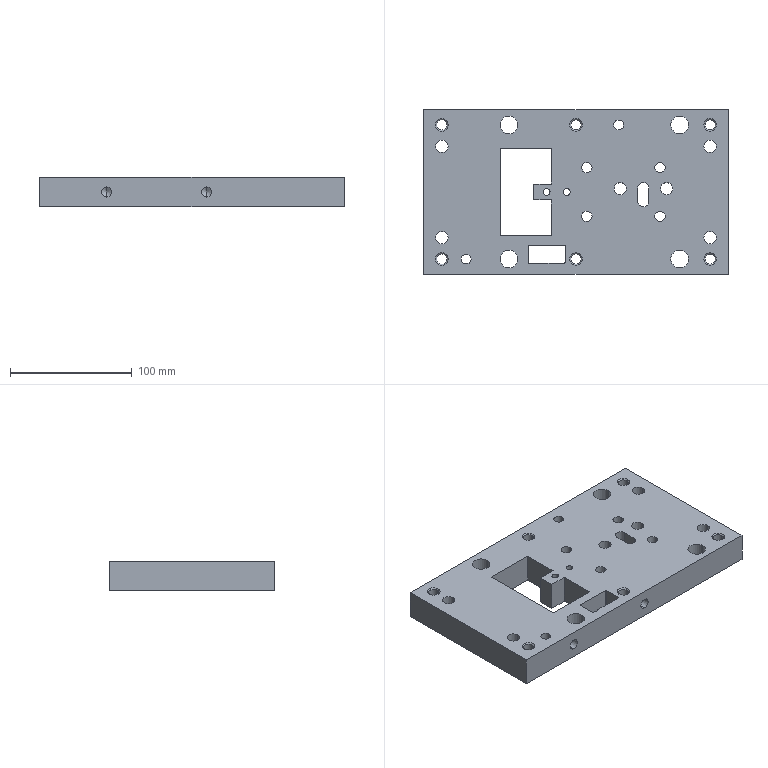Part | STEP file | MIENG DE KHUON AM KO LOGO | 1 solid | 126 faces | box 250 x 135 x 24 mm | volume 675291 mm3 | cylinder 71 | cone 28 | plane 27 | commonest cylinder face diameters 8.376 x16 8.5 x8 10 x8 10.106 x8 14 x8 14.5 x8